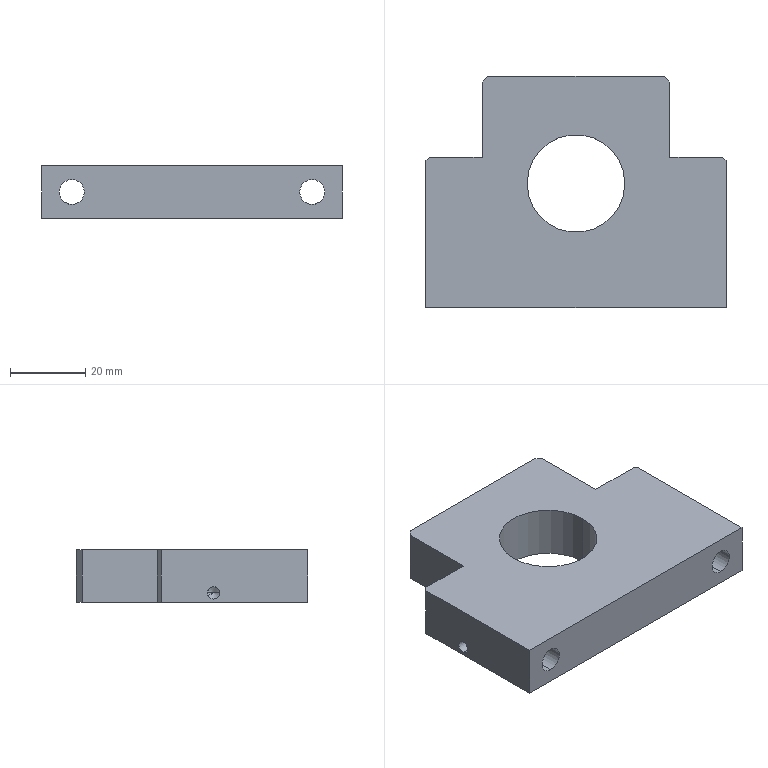Part | STEP file | 866-BDO024-93-03A | 1 solid | 42 faces | box 80 x 61.5 x 14 mm | volume 48551 mm3 | cylinder 18 | plane 16 | cone 8 | commonest cylinder face diameters 3.3 x8 6.6 x4 11 x4 26 x2
STEP:
#1=CARTESIAN_POINT('',(-13.,33.,7.));
#2=VERTEX_POINT('',#1);
#3=CARTESIAN_POINT('',(13.,33.,7.));
#4=VERTEX_POINT('',#3);
#5=CARTESIAN_POINT('',(0.,33.,7.));
#6=DIRECTION('',(0.,0.,1.));
#7=DIRECTION('',(-1.,0.,0.));
#8=AXIS2_PLACEMENT_3D('',#5,#6,#7);
#9=CIRCLE('',#8,13.);
#10=EDGE_CURVE('',#2,#4,#9,.T.);
#11=ORIENTED_EDGE('',*,*,#10,.T.);
#12=CARTESIAN_POINT('',(13.,33.,-7.));
#13=VERTEX_POINT('',#12);
#14=CARTESIAN_POINT('',(13.,33.,7.));
#15=DIRECTION('',(0.,0.,-1.));
#16=VECTOR('',#15,1000.);
#17=LINE('',#14,#16);
#18=EDGE_CURVE('',#4,#13,#17,.T.);
#19=ORIENTED_EDGE('',*,*,#18,.T.);
#20=CARTESIAN_POINT('',(-13.,33.,-7.));
#21=VERTEX_POINT('',#20);
#22=CARTESIAN_POINT('',(0.,33.,-7.));
#23=DIRECTION('',(0.,0.,1.));
#24=DIRECTION('',(-1.,0.,0.));
#25=AXIS2_PLACEMENT_3D('',#22,#23,#24);
#26=CIRCLE('',#25,13.);
#27=EDGE_CURVE('',#21,#13,#26,.T.);
#28=ORIENTED_EDGE('',*,*,#27,.F.);
#29=CARTESIAN_POINT('',(-13.,33.,7.));
#30=DIRECTION('',(0.,0.,-1.));
#31=VECTOR('',#30,1000.);
#32=LINE('',#29,#31);
#33=EDGE_CURVE('',#2,#21,#32,.T.);
#34=ORIENTED_EDGE('',*,*,#33,.F.);
#35=EDGE_LOOP('',(#11,#19,#28,#34));
#36=FACE_OUTER_BOUND('',#35,.T.);
#37=CARTESIAN_POINT('',(0.,33.,7.));
#38=DIRECTION('',(0.,0.,-1.));
#39=DIRECTION('',(-1.,0.,0.));
#40=AXIS2_PLACEMENT_3D('',#37,#38,#39);
#41=CYLINDRICAL_SURFACE('',#40,13.);
#42=ADVANCED_FACE('',(#36),#41,.F.);
#43=CARTESIAN_POINT('',(-15.,51.4,-1.65));
#44=VERTEX_POINT('',#43);
#45=CARTESIAN_POINT('',(-16.65,51.4,0.));
#46=VERTEX_POINT('',#45);
#47=CARTESIAN_POINT('',(-15.,51.4,0.));
#48=DIRECTION('',(0.,1.,0.));
#49=DIRECTION('',(0.,0.,1.));
#50=AXIS2_PLACEMENT_3D('',#47,#48,#49);
#51=CIRCLE('',#50,1.65);
#52=EDGE_CURVE('',#44,#46,#51,.T.);
#53=ORIENTED_EDGE('',*,*,#52,.F.);
#54=CARTESIAN_POINT('',(-15.,61.5,-1.65));
#55=VERTEX_POINT('',#54);
#56=CARTESIAN_POINT('',(-15.,61.5,-1.65));
#57=DIRECTION('',(0.,1.,0.));
#58=VECTOR('',#57,1000.);
#59=LINE('',#56,#58);
#60=EDGE_CURVE('',#44,#55,#59,.T.);
#61=ORIENTED_EDGE('',*,*,#60,.T.);
#62=CARTESIAN_POINT('',(-15.,61.5,1.65));
#63=VERTEX_POINT('',#62);
#64=CARTESIAN_POINT('',(-15.,61.5,0.));
#65=DIRECTION('',(0.,1.,0.));
#66=DIRECTION('',(0.,0.,1.));
#67=AXIS2_PLACEMENT_3D('',#64,#65,#66);
#68=CIRCLE('',#67,1.65);
#69=EDGE_CURVE('',#55,#63,#68,.T.);
#70=ORIENTED_EDGE('',*,*,#69,.T.);
#71=CARTESIAN_POINT('',(-15.,51.4,1.65));
#72=VERTEX_POINT('',#71);
#73=CARTESIAN_POINT('',(-15.,61.5,1.65));
#74=DIRECTION('',(0.,1.,0.));
#75=VECTOR('',#74,1000.);
#76=LINE('',#73,#75);
#77=EDGE_CURVE('',#72,#63,#76,.T.);
#78=ORIENTED_EDGE('',*,*,#77,.F.);
#79=CARTESIAN_POINT('',(-15.,51.4,0.));
#80=DIRECTION('',(0.,1.,0.));
#81=DIRECTION('',(0.,0.,1.));
#82=AXIS2_PLACEMENT_3D('',#79,#80,#81);
#83=CIRCLE('',#82,1.65);
#84=EDGE_CURVE('',#46,#72,#83,.T.);
#85=ORIENTED_EDGE('',*,*,#84,.F.);
#86=EDGE_LOOP('',(#53,#61,#70,#78,#85));
#87=FACE_OUTER_BOUND('',#86,.T.);
#88=CARTESIAN_POINT('',(-15.,61.5,0.));
#89=DIRECTION('',(0.,1.,0.));
#90=DIRECTION('',(0.,0.,1.));
#91=AXIS2_PLACEMENT_3D('',#88,#89,#90);
#92=CYLINDRICAL_SURFACE('',#91,1.65);
#93=ADVANCED_FACE('',(#87),#92,.F.);
#94=CARTESIAN_POINT('',(15.,51.4,-1.65));
#95=VERTEX_POINT('',#94);
#96=CARTESIAN_POINT('',(13.35,51.4,0.));
#97=VERTEX_POINT('',#96);
#98=CARTESIAN_POINT('',(15.,51.4,0.));
#99=DIRECTION('',(0.,1.,0.));
#100=DIRECTION('',(0.,0.,1.));
#101=AXIS2_PLACEMENT_3D('',#98,#99,#100);
#102=CIRCLE('',#101,1.65);
#103=EDGE_CURVE('',#95,#97,#102,.T.);
#104=ORIENTED_EDGE('',*,*,#103,.F.);
#105=CARTESIAN_POINT('',(15.,61.5,-1.65));
#106=VERTEX_POINT('',#105);
#107=CARTESIAN_POINT('',(15.,61.5,-1.65));
#108=DIRECTION('',(0.,1.,0.));
#109=VECTOR('',#108,1000.);
#110=LINE('',#107,#109);
#111=EDGE_CURVE('',#95,#106,#110,.T.);
#112=ORIENTED_EDGE('',*,*,#111,.T.);
#113=CARTESIAN_POINT('',(15.,61.5,1.65));
#114=VERTEX_POINT('',#113);
#115=CARTESIAN_POINT('',(15.,61.5,0.));
#116=DIRECTION('',(0.,1.,0.));
#117=DIRECTION('',(0.,0.,1.));
#118=AXIS2_PLACEMENT_3D('',#115,#116,#117);
#119=CIRCLE('',#118,1.65);
#120=EDGE_CURVE('',#106,#114,#119,.T.);
#121=ORIENTED_EDGE('',*,*,#120,.T.);
#122=CARTESIAN_POINT('',(15.,51.4,1.65));
#123=VERTEX_POINT('',#122);
#124=CARTESIAN_POINT('',(15.,61.5,1.65));
#125=DIRECTION('',(0.,1.,0.));
#126=VECTOR('',#125,1000.);
#127=LINE('',#124,#126);
#128=EDGE_CURVE('',#123,#114,#127,.T.);
#129=ORIENTED_EDGE('',*,*,#128,.F.);
#130=CARTESIAN_POINT('',(15.,51.4,0.));
#131=DIRECTION('',(0.,1.,0.));
#132=DIRECTION('',(0.,0.,1.));
#133=AXIS2_PLACEMENT_3D('',#130,#131,#132);
#134=CIRCLE('',#133,1.65);
#135=EDGE_CURVE('',#97,#123,#134,.T.);
#136=ORIENTED_EDGE('',*,*,#135,.F.);
#137=EDGE_LOOP('',(#104,#112,#121,#129,#136));
#138=FACE_OUTER_BOUND('',#137,.T.);
#139=CARTESIAN_POINT('',(15.,61.5,0.));
#140=DIRECTION('',(0.,1.,0.));
#141=DIRECTION('',(0.,0.,1.));
#142=AXIS2_PLACEMENT_3D('',#139,#140,#141);
#143=CYLINDRICAL_SURFACE('',#142,1.65);
#144=ADVANCED_FACE('',(#138),#143,.F.);
#145=CARTESIAN_POINT('',(-32.,34.,-5.5));
#146=VERTEX_POINT('',#145);
#147=CARTESIAN_POINT('',(-32.,34.,5.5));
#148=VERTEX_POINT('',#147);
#149=CARTESIAN_POINT('',(-32.,34.,0.));
#150=DIRECTION('',(0.,1.,0.));
#151=DIRECTION('',(0.,0.,1.));
#152=AXIS2_PLACEMENT_3D('',#149,#150,#151);
#153=CIRCLE('',#152,5.5);
#154=EDGE_CURVE('',#146,#148,#153,.T.);
#155=ORIENTED_EDGE('',*,*,#154,.F.);
#156=CARTESIAN_POINT('',(-32.,40.,-5.5));
#157=VERTEX_POINT('',#156);
#158=CARTESIAN_POINT('',(-32.,40.,-5.5));
#159=DIRECTION('',(0.,1.,0.));
#160=VECTOR('',#159,1000.);
#161=LINE('',#158,#160);
#162=EDGE_CURVE('',#146,#157,#161,.T.);
#163=ORIENTED_EDGE('',*,*,#162,.T.);
#164=CARTESIAN_POINT('',(-32.,40.,5.5));
#165=VERTEX_POINT('',#164);
#166=CARTESIAN_POINT('',(-32.,40.,0.));
#167=DIRECTION('',(0.,1.,0.));
#168=DIRECTION('',(0.,0.,1.));
#169=AXIS2_PLACEMENT_3D('',#166,#167,#168);
#170=CIRCLE('',#169,5.5);
#171=EDGE_CURVE('',#157,#165,#170,.T.);
#172=ORIENTED_EDGE('',*,*,#171,.T.);
#173=CARTESIAN_POINT('',(-32.,40.,5.5));
#174=DIRECTION('',(0.,1.,0.));
#175=VECTOR('',#174,1000.);
#176=LINE('',#173,#175);
#177=EDGE_CURVE('',#148,#165,#176,.T.);
#178=ORIENTED_EDGE('',*,*,#177,.F.);
#179=EDGE_LOOP('',(#155,#163,#172,#178));
#180=FACE_OUTER_BOUND('',#179,.T.);
#181=CARTESIAN_POINT('',(-32.,40.,0.));
#182=DIRECTION('',(0.,1.,0.));
#183=DIRECTION('',(0.,0.,1.));
#184=AXIS2_PLACEMENT_3D('',#181,#182,#183);
#185=CYLINDRICAL_SURFACE('',#184,5.5);
#186=ADVANCED_FACE('',(#180),#185,.F.);
#187=CARTESIAN_POINT('',(-29.9,25.,-6.15));
#188=VERTEX_POINT('',#187);
#189=CARTESIAN_POINT('',(-29.9,23.35,-4.5));
#190=VERTEX_POINT('',#189);
#191=CARTESIAN_POINT('',(-29.9,25.,-4.5));
#192=DIRECTION('',(-1.,0.,0.));
#193=DIRECTION('',(0.,0.,1.));
#194=AXIS2_PLACEMENT_3D('',#191,#192,#193);
#195=CIRCLE('',#194,1.65);
#196=EDGE_CURVE('',#188,#190,#195,.T.);
#197=ORIENTED_EDGE('',*,*,#196,.F.);
#198=CARTESIAN_POINT('',(-40.,25.,-6.15));
#199=VERTEX_POINT('',#198);
#200=CARTESIAN_POINT('',(-40.,25.,-6.15));
#201=DIRECTION('',(-1.,0.,0.));
#202=VECTOR('',#201,1000.);
#203=LINE('',#200,#202);
#204=EDGE_CURVE('',#188,#199,#203,.T.);
#205=ORIENTED_EDGE('',*,*,#204,.T.);
#206=CARTESIAN_POINT('',(-40.,25.,-2.85));
#207=VERTEX_POINT('',#206);
#208=CARTESIAN_POINT('',(-40.,25.,-4.5));
#209=DIRECTION('',(-1.,0.,0.));
#210=DIRECTION('',(0.,0.,1.));
#211=AXIS2_PLACEMENT_3D('',#208,#209,#210);
#212=CIRCLE('',#211,1.65);
#213=EDGE_CURVE('',#199,#207,#212,.T.);
#214=ORIENTED_EDGE('',*,*,#213,.T.);
#215=CARTESIAN_POINT('',(-33.664,25.,-2.85));
#216=VERTEX_POINT('',#215);
#217=CARTESIAN_POINT('',(-40.,25.,-2.85));
#218=DIRECTION('',(-1.,0.,0.));
#219=VECTOR('',#218,1000.);
#220=LINE('',#217,#219);
#221=EDGE_CURVE('',#216,#207,#220,.T.);
#222=ORIENTED_EDGE('',*,*,#221,.F.);
#223=CARTESIAN_POINT('',(-32.,23.868,-3.3));
#224=VERTEX_POINT('',#223);
#225=CARTESIAN_POINT('',(-32.,23.868,-3.3));
#226=CARTESIAN_POINT('',(-32.193,23.868,-3.3));
#227=CARTESIAN_POINT('',(-32.381,23.885,-3.283));
#228=CARTESIAN_POINT('',(-32.748,23.958,-3.219));
#229=CARTESIAN_POINT('',(-32.929,24.016,-3.171));
#230=CARTESIAN_POINT('',(-33.251,24.191,-3.058));
#231=CARTESIAN_POINT('',(-33.395,24.308,-2.993));
#232=CARTESIAN_POINT('',(-33.604,24.618,-2.886));
#233=CARTESIAN_POINT('',(-33.664,24.805,-2.85));
#234=CARTESIAN_POINT('',(-33.664,25.,-2.85));
#235=B_SPLINE_CURVE_WITH_KNOTS('',3,(#225,#226,#227,#228,#229,#230,#231,#232,#233,#234),.UNSPECIFIED.,.F.,.F.,(4,2,2,2,4),(0.004543,0.005111,0.005678,0.006246,0.006814),.UNSPECIFIED.);
#236=EDGE_CURVE('',#224,#216,#235,.T.);
#237=ORIENTED_EDGE('',*,*,#236,.F.);
#238=CARTESIAN_POINT('',(-30.336,25.,-2.85));
#239=VERTEX_POINT('',#238);
#240=CARTESIAN_POINT('',(-30.336,25.,-2.85));
#241=CARTESIAN_POINT('',(-30.336,24.903,-2.85));
#242=CARTESIAN_POINT('',(-30.351,24.809,-2.859));
#243=CARTESIAN_POINT('',(-30.407,24.627,-2.89));
#244=CARTESIAN_POINT('',(-30.448,24.542,-2.913));
#245=CARTESIAN_POINT('',(-30.603,24.311,-2.992));
#246=CARTESIAN_POINT('',(-30.747,24.192,-3.057));
#247=CARTESIAN_POINT('',(-31.069,24.017,-3.171));
#248=CARTESIAN_POINT('',(-31.247,23.959,-3.219));
#249=CARTESIAN_POINT('',(-31.618,23.884,-3.283));
#250=CARTESIAN_POINT('',(-31.807,23.868,-3.3));
#251=CARTESIAN_POINT('',(-32.,23.868,-3.3));
#252=B_SPLINE_CURVE_WITH_KNOTS('',3,(#240,#241,#242,#243,#244,#245,#246,#247,#248,#249,#250,#251),.UNSPECIFIED.,.F.,.F.,(4,2,2,2,2,4),(0.002272,0.002556,0.00284,0.003408,0.003975,0.004543),.UNSPECIFIED.);
#253=EDGE_CURVE('',#239,#224,#252,.T.);
#254=ORIENTED_EDGE('',*,*,#253,.F.);
#255=CARTESIAN_POINT('',(-29.9,25.,-2.85));
#256=VERTEX_POINT('',#255);
#257=CARTESIAN_POINT('',(-40.,25.,-2.85));
#258=DIRECTION('',(-1.,0.,0.));
#259=VECTOR('',#258,1000.);
#260=LINE('',#257,#259);
#261=EDGE_CURVE('',#256,#239,#260,.T.);
#262=ORIENTED_EDGE('',*,*,#261,.F.);
#263=CARTESIAN_POINT('',(-29.9,25.,-4.5));
#264=DIRECTION('',(-1.,0.,0.));
#265=DIRECTION('',(0.,0.,1.));
#266=AXIS2_PLACEMENT_3D('',#263,#264,#265);
#267=CIRCLE('',#266,1.65);
#268=EDGE_CURVE('',#190,#256,#267,.T.);
#269=ORIENTED_EDGE('',*,*,#268,.F.);
#270=EDGE_LOOP('',(#197,#205,#214,#222,#237,#254,#262,#269));
#271=FACE_OUTER_BOUND('',#270,.T.);
#272=CARTESIAN_POINT('',(-40.,25.,-4.5));
#273=DIRECTION('',(-1.,0.,0.));
#274=DIRECTION('',(0.,0.,1.));
#275=AXIS2_PLACEMENT_3D('',#272,#273,#274);
#276=CYLINDRICAL_SURFACE('',#275,1.65);
#277=ADVANCED_FACE('',(#271),#276,.F.);
#278=CARTESIAN_POINT('',(-32.,0.,3.3));
#279=VERTEX_POINT('',#278);
#280=CARTESIAN_POINT('',(-32.,0.,-3.3));
#281=VERTEX_POINT('',#280);
#282=CARTESIAN_POINT('',(-32.,0.,0.));
#283=DIRECTION('',(0.,-1.,0.));
#284=DIRECTION('',(0.,0.,1.));
#285=AXIS2_PLACEMENT_3D('',#282,#283,#284);
#286=CIRCLE('',#285,3.3);
#287=EDGE_CURVE('',#279,#281,#286,.T.);
#288=ORIENTED_EDGE('',*,*,#287,.T.);
#289=CARTESIAN_POINT('',(-32.,40.,-3.3));
#290=DIRECTION('',(0.,1.,0.));
#291=VECTOR('',#290,1000.);
#292=LINE('',#289,#291);
#293=EDGE_CURVE('',#281,#224,#292,.T.);
#294=ORIENTED_EDGE('',*,*,#293,.T.);
#295=ORIENTED_EDGE('',*,*,#236,.T.);
#296=CARTESIAN_POINT('',(-32.,26.132,-3.3));
#297=VERTEX_POINT('',#296);
#298=CARTESIAN_POINT('',(-33.664,25.,-2.85));
#299=CARTESIAN_POINT('',(-33.664,25.097,-2.85));
#300=CARTESIAN_POINT('',(-33.649,25.191,-2.859));
#301=CARTESIAN_POINT('',(-33.593,25.373,-2.89));
#302=CARTESIAN_POINT('',(-33.552,25.458,-2.913));
#303=CARTESIAN_POINT('',(-33.397,25.689,-2.992));
#304=CARTESIAN_POINT('',(-33.253,25.808,-3.057));
#305=CARTESIAN_POINT('',(-32.931,25.983,-3.171));
#306=CARTESIAN_POINT('',(-32.753,26.041,-3.219));
#307=CARTESIAN_POINT('',(-32.382,26.116,-3.283));
#308=CARTESIAN_POINT('',(-32.193,26.132,-3.3));
#309=CARTESIAN_POINT('',(-32.,26.132,-3.3));
#310=B_SPLINE_CURVE_WITH_KNOTS('',3,(#298,#299,#300,#301,#302,#303,#304,#305,#306,#307,#308,#309),.UNSPECIFIED.,.F.,.F.,(4,2,2,2,2,4),(-0.002271,-0.001987,-0.001703,-0.001136,-0.0005678,0.),.UNSPECIFIED.);
#311=EDGE_CURVE('',#216,#297,#310,.T.);
#312=ORIENTED_EDGE('',*,*,#311,.T.);
#313=CARTESIAN_POINT('',(-32.,34.,-3.3));
#314=VERTEX_POINT('',#313);
#315=CARTESIAN_POINT('',(-32.,40.,-3.3));
#316=DIRECTION('',(0.,1.,0.));
#317=VECTOR('',#316,1000.);
#318=LINE('',#315,#317);
#319=EDGE_CURVE('',#297,#314,#318,.T.);
#320=ORIENTED_EDGE('',*,*,#319,.T.);
#321=CARTESIAN_POINT('',(-32.,34.,3.3));
#322=VERTEX_POINT('',#321);
#323=CARTESIAN_POINT('',(-32.,34.,0.));
#324=DIRECTION('',(0.,-1.,0.));
#325=DIRECTION('',(0.,0.,1.));
#326=AXIS2_PLACEMENT_3D('',#323,#324,#325);
#327=CIRCLE('',#326,3.3);
#328=EDGE_CURVE('',#322,#314,#327,.T.);
#329=ORIENTED_EDGE('',*,*,#328,.F.);
#330=CARTESIAN_POINT('',(-32.,40.,3.3));
#331=DIRECTION('',(0.,1.,0.));
#332=VECTOR('',#331,1000.);
#333=LINE('',#330,#332);
#334=EDGE_CURVE('',#279,#322,#333,.T.);
#335=ORIENTED_EDGE('',*,*,#334,.F.);
#336=EDGE_LOOP('',(#288,#294,#295,#312,#320,#329,#335));
#337=FACE_OUTER_BOUND('',#336,.T.);
#338=CARTESIAN_POINT('',(-32.,40.,0.));
#339=DIRECTION('',(0.,1.,0.));
#340=DIRECTION('',(0.,0.,1.));
#341=AXIS2_PLACEMENT_3D('',#338,#339,#340);
#342=CYLINDRICAL_SURFACE('',#341,3.3);
#343=ADVANCED_FACE('',(#337),#342,.F.);
#344=CARTESIAN_POINT('',(32.,0.,3.3));
#345=VERTEX_POINT('',#344);
#346=CARTESIAN_POINT('',(32.,0.,-3.3));
#347=VERTEX_POINT('',#346);
#348=CARTESIAN_POINT('',(32.,0.,0.));
#349=DIRECTION('',(0.,-1.,0.));
#350=DIRECTION('',(0.,0.,1.));
#351=AXIS2_PLACEMENT_3D('',#348,#349,#350);
#352=CIRCLE('',#351,3.3);
#353=EDGE_CURVE('',#345,#347,#352,.T.);
#354=ORIENTED_EDGE('',*,*,#353,.T.);
#355=CARTESIAN_POINT('',(32.,23.868,-3.3));
#356=VERTEX_POINT('',#355);
#357=CARTESIAN_POINT('',(32.,40.,-3.3));
#358=DIRECTION('',(0.,1.,0.));
#359=VECTOR('',#358,1000.);
#360=LINE('',#357,#359);
#361=EDGE_CURVE('',#347,#356,#360,.T.);
#362=ORIENTED_EDGE('',*,*,#361,.T.);
#363=CARTESIAN_POINT('',(30.336,25.,-2.85));
#364=VERTEX_POINT('',#363);
#365=CARTESIAN_POINT('',(30.336,25.,-2.85));
#366=CARTESIAN_POINT('',(30.336,24.903,-2.85));
#367=CARTESIAN_POINT('',(30.351,24.809,-2.859));
#368=CARTESIAN_POINT('',(30.407,24.627,-2.89));
#369=CARTESIAN_POINT('',(30.448,24.542,-2.913));
#370=CARTESIAN_POINT('',(30.603,24.311,-2.992));
#371=CARTESIAN_POINT('',(30.747,24.192,-3.057));
#372=CARTESIAN_POINT('',(31.069,24.017,-3.171));
#373=CARTESIAN_POINT('',(31.247,23.959,-3.219));
#374=CARTESIAN_POINT('',(31.618,23.884,-3.283));
#375=CARTESIAN_POINT('',(31.807,23.868,-3.3));
#376=CARTESIAN_POINT('',(32.,23.868,-3.3));
#377=B_SPLINE_CURVE_WITH_KNOTS('',3,(#365,#366,#367,#368,#369,#370,#371,#372,#373,#374,#375,#376),.UNSPECIFIED.,.F.,.F.,(4,2,2,2,2,4),(0.004583,0.004869,0.005155,0.005728,0.0063,0.006873),.UNSPECIFIED.);
#378=EDGE_CURVE('',#364,#356,#377,.T.);
#379=ORIENTED_EDGE('',*,*,#378,.F.);
#380=CARTESIAN_POINT('',(32.,26.132,-3.3));
#381=VERTEX_POINT('',#380);
#382=CARTESIAN_POINT('',(32.,26.132,-3.3));
#383=CARTESIAN_POINT('',(31.807,26.132,-3.3));
#384=CARTESIAN_POINT('',(31.619,26.115,-3.283));
#385=CARTESIAN_POINT('',(31.252,26.042,-3.219));
#386=CARTESIAN_POINT('',(31.071,25.984,-3.171));
#387=CARTESIAN_POINT('',(30.749,25.809,-3.058));
#388=CARTESIAN_POINT('',(30.605,25.692,-2.993));
#389=CARTESIAN_POINT('',(30.396,25.382,-2.886));
#390=CARTESIAN_POINT('',(30.336,25.195,-2.85));
#391=CARTESIAN_POINT('',(30.336,25.,-2.85));
#392=B_SPLINE_CURVE_WITH_KNOTS('',3,(#382,#383,#384,#385,#386,#387,#388,#389,#390,#391),.UNSPECIFIED.,.F.,.F.,(4,2,2,2,4),(0.002291,0.002864,0.003437,0.00401,0.004583),.UNSPECIFIED.);
#393=EDGE_CURVE('',#381,#364,#392,.T.);
#394=ORIENTED_EDGE('',*,*,#393,.F.);
#395=CARTESIAN_POINT('',(32.,34.,-3.3));
#396=VERTEX_POINT('',#395);
#397=CARTESIAN_POINT('',(32.,40.,-3.3));
#398=DIRECTION('',(0.,1.,0.));
#399=VECTOR('',#398,1000.);
#400=LINE('',#397,#399);
#401=EDGE_CURVE('',#381,#396,#400,.T.);
#402=ORIENTED_EDGE('',*,*,#401,.T.);
#403=CARTESIAN_POINT('',(32.,34.,3.3));
#404=VERTEX_POINT('',#403);
#405=CARTESIAN_POINT('',(32.,34.,0.));
#406=DIRECTION('',(0.,-1.,0.));
#407=DIRECTION('',(0.,0.,1.));
#408=AXIS2_PLACEMENT_3D('',#405,#406,#407);
#409=CIRCLE('',#408,3.3);
#410=EDGE_CURVE('',#404,#396,#409,.T.);
#411=ORIENTED_EDGE('',*,*,#410,.F.);
#412=CARTESIAN_POINT('',(32.,40.,3.3));
#413=DIRECTION('',(0.,1.,0.));
#414=VECTOR('',#413,1000.);
#415=LINE('',#412,#414);
#416=EDGE_CURVE('',#345,#404,#415,.T.);
#417=ORIENTED_EDGE('',*,*,#416,.F.);
#418=EDGE_LOOP('',(#354,#362,#379,#394,#402,#411,#417));
#419=FACE_OUTER_BOUND('',#418,.T.);
#420=CARTESIAN_POINT('',(32.,40.,0.));
#421=DIRECTION('',(0.,1.,0.));
#422=DIRECTION('',(0.,0.,1.));
#423=AXIS2_PLACEMENT_3D('',#420,#421,#422);
#424=CYLINDRICAL_SURFACE('',#423,3.3);
#425=ADVANCED_FACE('',(#419),#424,.F.);
#426=CARTESIAN_POINT('',(29.9,25.,-2.85));
#427=VERTEX_POINT('',#426);
#428=CARTESIAN_POINT('',(29.9,25.,-6.15));
#429=VERTEX_POINT('',#428);
#430=CARTESIAN_POINT('',(29.9,25.,-4.5));
#431=DIRECTION('',(1.,0.,0.));
#432=DIRECTION('',(0.,0.,-1.));
#433=AXIS2_PLACEMENT_3D('',#430,#431,#432);
#434=CIRCLE('',#433,1.65);
#435=EDGE_CURVE('',#427,#429,#434,.T.);
#436=ORIENTED_EDGE('',*,*,#435,.F.);
#437=CARTESIAN_POINT('',(40.,25.,-2.85));
#438=DIRECTION('',(1.,0.,0.));
#439=VECTOR('',#438,1000.);
#440=LINE('',#437,#439);
#441=EDGE_CURVE('',#427,#364,#440,.T.);
#442=ORIENTED_EDGE('',*,*,#441,.T.);
#443=ORIENTED_EDGE('',*,*,#378,.T.);
#444=CARTESIAN_POINT('',(33.664,25.,-2.85));
#445=VERTEX_POINT('',#444);
#446=CARTESIAN_POINT('',(32.,23.868,-3.3));
#447=CARTESIAN_POINT('',(32.193,23.868,-3.3));
#448=CARTESIAN_POINT('',(32.381,23.885,-3.283));
#449=CARTESIAN_POINT('',(32.748,23.958,-3.219));
#450=CARTESIAN_POINT('',(32.929,24.016,-3.171));
#451=CARTESIAN_POINT('',(33.251,24.191,-3.058));
#452=CARTESIAN_POINT('',(33.395,24.308,-2.993));
#453=CARTESIAN_POINT('',(33.604,24.618,-2.886));
#454=CARTESIAN_POINT('',(33.664,24.805,-2.85));
#455=CARTESIAN_POINT('',(33.664,25.,-2.85));
#456=B_SPLINE_CURVE_WITH_KNOTS('',3,(#446,#447,#448,#449,#450,#451,#452,#453,#454,#455),.UNSPECIFIED.,.F.,.F.,(4,2,2,2,4),(-0.002293,-0.00172,-0.001146,-0.0005732,0.),.UNSPECIFIED.);
#457=EDGE_CURVE('',#356,#445,#456,.T.);
#458=ORIENTED_EDGE('',*,*,#457,.T.);
#459=CARTESIAN_POINT('',(40.,25.,-2.85));
#460=VERTEX_POINT('',#459);
#461=CARTESIAN_POINT('',(40.,25.,-2.85));
#462=DIRECTION('',(1.,0.,0.));
#463=VECTOR('',#462,1000.);
#464=LINE('',#461,#463);
#465=EDGE_CURVE('',#445,#460,#464,.T.);
#466=ORIENTED_EDGE('',*,*,#465,.T.);
#467=CARTESIAN_POINT('',(40.,25.,-6.15));
#468=VERTEX_POINT('',#467);
#469=CARTESIAN_POINT('',(40.,25.,-4.5));
#470=DIRECTION('',(1.,0.,0.));
#471=DIRECTION('',(0.,0.,-1.));
#472=AXIS2_PLACEMENT_3D('',#469,#470,#471);
#473=CIRCLE('',#472,1.65);
#474=EDGE_CURVE('',#460,#468,#473,.T.);
#475=ORIENTED_EDGE('',*,*,#474,.T.);
#476=CARTESIAN_POINT('',(40.,25.,-6.15));
#477=DIRECTION('',(1.,0.,0.));
#478=VECTOR('',#477,1000.);
#479=LINE('',#476,#478);
#480=EDGE_CURVE('',#429,#468,#479,.T.);
#481=ORIENTED_EDGE('',*,*,#480,.F.);
#482=EDGE_LOOP('',(#436,#442,#443,#458,#466,#475,#481));
#483=FACE_OUTER_BOUND('',#482,.T.);
#484=CARTESIAN_POINT('',(40.,25.,-4.5));
#485=DIRECTION('',(1.,0.,0.));
#486=DIRECTION('',(0.,0.,-1.));
#487=AXIS2_PLACEMENT_3D('',#484,#485,#486);
#488=CYLINDRICAL_SURFACE('',#487,1.65);
#489=ADVANCED_FACE('',(#483),#488,.F.);
#490=CARTESIAN_POINT('',(32.,34.,-5.5));
#491=VERTEX_POINT('',#490);
#492=CARTESIAN_POINT('',(32.,34.,5.5));
#493=VERTEX_POINT('',#492);
#494=CARTESIAN_POINT('',(32.,34.,0.));
#495=DIRECTION('',(0.,1.,0.));
#496=DIRECTION('',(0.,0.,1.));
#497=AXIS2_PLACEMENT_3D('',#494,#495,#496);
#498=CIRCLE('',#497,5.5);
#499=EDGE_CURVE('',#491,#493,#498,.T.);
#500=ORIENTED_EDGE('',*,*,#499,.F.);
#501=CARTESIAN_POINT('',(32.,40.,-5.5));
#502=VERTEX_POINT('',#501);
#503=CARTESIAN_POINT('',(32.,40.,-5.5));
#504=DIRECTION('',(0.,1.,0.));
#505=VECTOR('',#504,1000.);
#506=LINE('',#503,#505);
#507=EDGE_CURVE('',#491,#502,#506,.T.);
#508=ORIENTED_EDGE('',*,*,#507,.T.);
#509=CARTESIAN_POINT('',(32.,40.,5.5));
#510=VERTEX_POINT('',#509);
#511=CARTESIAN_POINT('',(32.,40.,0.));
#512=DIRECTION('',(0.,1.,0.));
#513=DIRECTION('',(0.,0.,1.));
#514=AXIS2_PLACEMENT_3D('',#511,#512,#513);
#515=CIRCLE('',#514,5.5);
#516=EDGE_CURVE('',#502,#510,#515,.T.);
#517=ORIENTED_EDGE('',*,*,#516,.T.);
#518=CARTESIAN_POINT('',(32.,40.,5.5));
#519=DIRECTION('',(0.,1.,0.));
#520=VECTOR('',#519,1000.);
#521=LINE('',#518,#520);
#522=EDGE_CURVE('',#493,#510,#521,.T.);
#523=ORIENTED_EDGE('',*,*,#522,.F.);
#524=EDGE_LOOP('',(#500,#508,#517,#523));
#525=FACE_OUTER_BOUND('',#524,.T.);
#526=CARTESIAN_POINT('',(32.,40.,0.));
#527=DIRECTION('',(0.,1.,0.));
#528=DIRECTION('',(0.,0.,1.));
#529=AXIS2_PLACEMENT_3D('',#526,#527,#528);
#530=CYLINDRICAL_SURFACE('',#529,5.5);
#531=ADVANCED_FACE('',(#525),#530,.F.);
#532=CARTESIAN_POINT('',(-15.,50.409,0.));
#533=VERTEX_POINT('',#532);
#534=CARTESIAN_POINT('',(-16.65,51.4,0.));
#535=DIRECTION('',(-0.8572,0.515,0.));
#536=VECTOR('',#535,1000.);
#537=LINE('',#534,#536);
#538=EDGE_CURVE('',#533,#46,#537,.T.);
#539=ORIENTED_EDGE('',*,*,#538,.F.);
#540=CARTESIAN_POINT('',(-13.35,51.4,0.));
#541=VERTEX_POINT('',#540);
#542=CARTESIAN_POINT('',(-13.35,51.4,0.));
#543=DIRECTION('',(0.8572,0.515,0.));
#544=VECTOR('',#543,1000.);
#545=LINE('',#542,#544);
#546=EDGE_CURVE('',#533,#541,#545,.T.);
#547=ORIENTED_EDGE('',*,*,#546,.T.);
#548=CARTESIAN_POINT('',(-15.,51.4,0.));
#549=DIRECTION('',(0.,1.,0.));
#550=DIRECTION('',(0.,0.,1.));
#551=AXIS2_PLACEMENT_3D('',#548,#549,#550);
#552=CIRCLE('',#551,1.65);
#553=EDGE_CURVE('',#541,#44,#552,.T.);
#554=ORIENTED_EDGE('',*,*,#553,.T.);
#555=ORIENTED_EDGE('',*,*,#52,.T.);
#556=EDGE_LOOP('',(#539,#547,#554,#555));
#557=FACE_OUTER_BOUND('',#556,.T.);
#558=CARTESIAN_POINT('',(-15.,51.4,0.));
#559=DIRECTION('',(0.,1.,0.));
#560=DIRECTION('',(-1.,0.,0.));
#561=AXIS2_PLACEMENT_3D('',#558,#559,#560);
#562=CONICAL_SURFACE('',#561,1.65,1.03);
#563=ADVANCED_FACE('',(#557),#562,.F.);
#564=CARTESIAN_POINT('',(15.,50.409,0.));
#565=VERTEX_POINT('',#564);
#566=CARTESIAN_POINT('',(13.35,51.4,0.));
#567=DIRECTION('',(-0.8572,0.515,0.));
#568=VECTOR('',#567,1000.);
#569=LINE('',#566,#568);
#570=EDGE_CURVE('',#565,#97,#569,.T.);
#571=ORIENTED_EDGE('',*,*,#570,.F.);
#572=CARTESIAN_POINT('',(16.65,51.4,0.));
#573=VERTEX_POINT('',#572);
#574=CARTESIAN_POINT('',(16.65,51.4,0.));
#575=DIRECTION('',(0.8572,0.515,0.));
#576=VECTOR('',#575,1000.);
#577=LINE('',#574,#576);
#578=EDGE_CURVE('',#565,#573,#577,.T.);
#579=ORIENTED_EDGE('',*,*,#578,.T.);
#580=CARTESIAN_POINT('',(15.,51.4,0.));
#581=DIRECTION('',(0.,1.,0.));
#582=DIRECTION('',(0.,0.,1.));
#583=AXIS2_PLACEMENT_3D('',#580,#581,#582);
#584=CIRCLE('',#583,1.65);
#585=EDGE_CURVE('',#573,#95,#584,.T.);
#586=ORIENTED_EDGE('',*,*,#585,.T.);
#587=ORIENTED_EDGE('',*,*,#103,.T.);
#588=EDGE_LOOP('',(#571,#579,#586,#587));
#589=FACE_OUTER_BOUND('',#588,.T.);
#590=CARTESIAN_POINT('',(15.,51.4,0.));
#591=DIRECTION('',(0.,1.,0.));
#592=DIRECTION('',(-1.,0.,0.));
#593=AXIS2_PLACEMENT_3D('',#590,#591,#592);
#594=CONICAL_SURFACE('',#593,1.65,1.03);
#595=ADVANCED_FACE('',(#589),#594,.F.);
#596=CARTESIAN_POINT('',(-28.909,25.,-4.5));
#597=VERTEX_POINT('',#596);
#598=CARTESIAN_POINT('',(-29.9,23.35,-4.5));
#599=DIRECTION('',(-0.515,-0.8572,0.));
#600=VECTOR('',#599,1000.);
#601=LINE('',#598,#600);
#602=EDGE_CURVE('',#597,#190,#601,.T.);
#603=ORIENTED_EDGE('',*,*,#602,.F.);
#604=CARTESIAN_POINT('',(-29.9,26.65,-4.5));
#605=VERTEX_POINT('',#604);
#606=CARTESIAN_POINT('',(-29.9,26.65,-4.5));
#607=DIRECTION('',(-0.515,0.8572,0.));
#608=VECTOR('',#607,1000.);
#609=LINE('',#606,#608);
#610=EDGE_CURVE('',#597,#605,#609,.T.);
#611=ORIENTED_EDGE('',*,*,#610,.T.);
#612=CARTESIAN_POINT('',(-29.9,25.,-4.5));
#613=DIRECTION('',(-1.,0.,0.));
#614=DIRECTION('',(0.,0.,1.));
#615=AXIS2_PLACEMENT_3D('',#612,#613,#614);
#616=CIRCLE('',#615,1.65);
#617=EDGE_CURVE('',#605,#188,#616,.T.);
#618=ORIENTED_EDGE('',*,*,#617,.T.);
#619=ORIENTED_EDGE('',*,*,#196,.T.);
#620=EDGE_LOOP('',(#603,#611,#618,#619));
#621=FACE_OUTER_BOUND('',#620,.T.);
#622=CARTESIAN_POINT('',(-29.9,25.,-4.5));
#623=DIRECTION('',(-1.,0.,0.));
#624=DIRECTION('',(0.,-1.,0.));
#625=AXIS2_PLACEMENT_3D('',#622,#623,#624);
#626=CONICAL_SURFACE('',#625,1.65,1.03);
#627=ADVANCED_FACE('',(#621),#626,.F.);
#628=CARTESIAN_POINT('',(28.909,25.,-4.5));
#629=VERTEX_POINT('',#628);
#630=CARTESIAN_POINT('',(29.9,25.,-6.15));
#631=DIRECTION('',(0.515,0.,-0.8572));
#632=VECTOR('',#631,1000.);
#633=LINE('',#630,#632);
#634=EDGE_CURVE('',#629,#429,#633,.T.);
#635=ORIENTED_EDGE('',*,*,#634,.F.);
#636=CARTESIAN_POINT('',(29.9,25.,-2.85));
#637=DIRECTION('',(0.515,0.,0.8572));
#638=VECTOR('',#637,1000.);
#639=LINE('',#636,#638);
#640=EDGE_CURVE('',#629,#427,#639,.T.);
#641=ORIENTED_EDGE('',*,*,#640,.T.);
#642=ORIENTED_EDGE('',*,*,#435,.T.);
#643=EDGE_LOOP('',(#635,#641,#642));
#644=FACE_OUTER_BOUND('',#643,.T.);
#645=CARTESIAN_POINT('',(29.9,25.,-4.5));
#646=DIRECTION('',(1.,0.,0.));
#647=DIRECTION('',(0.,0.,-1.));
#648=AXIS2_PLACEMENT_3D('',#645,#646,#647);
#649=CONICAL_SURFACE('',#648,1.65,1.03);
#650=ADVANCED_FACE('',(#644),#649,.F.);
#651=ORIENTED_EDGE('',*,*,#10,.F.);
#652=CARTESIAN_POINT('',(0.,33.,7.));
#653=DIRECTION('',(0.,0.,1.));
#654=DIRECTION('',(-1.,0.,0.));
#655=AXIS2_PLACEMENT_3D('',#652,#653,#654);
#656=CIRCLE('',#655,13.);
#657=EDGE_CURVE('',#4,#2,#656,.T.);
#658=ORIENTED_EDGE('',*,*,#657,.F.);
#659=EDGE_LOOP('',(#651,#658));
#660=FACE_BOUND('',#659,.T.);
#661=CARTESIAN_POINT('',(23.5,61.5,7.));
#662=VERTEX_POINT('',#661);
#663=CARTESIAN_POINT('',(25.,60.,7.));
#664=VERTEX_POINT('',#663);
#665=CARTESIAN_POINT('',(23.5,61.5,7.));
#666=DIRECTION('',(0.7071,-0.7071,0.));
#667=VECTOR('',#666,1000.);
#668=LINE('',#665,#667);
#669=EDGE_CURVE('',#662,#664,#668,.T.);
#670=ORIENTED_EDGE('',*,*,#669,.F.);
#671=CARTESIAN_POINT('',(-23.5,61.5,7.));
#672=VERTEX_POINT('',#671);
#673=CARTESIAN_POINT('',(-40.,61.5,7.));
#674=DIRECTION('',(1.,0.,0.));
#675=VECTOR('',#674,1000.);
#676=LINE('',#673,#675);
#677=EDGE_CURVE('',#672,#662,#676,.T.);
#678=ORIENTED_EDGE('',*,*,#677,.F.);
#679=CARTESIAN_POINT('',(-25.,60.,7.));
#680=VERTEX_POINT('',#679);
#681=CARTESIAN_POINT('',(-25.,60.,7.));
#682=DIRECTION('',(0.7071,0.7071,0.));
#683=VECTOR('',#682,1000.);
#684=LINE('',#681,#683);
#685=EDGE_CURVE('',#680,#672,#684,.T.);
#686=ORIENTED_EDGE('',*,*,#685,.F.);
#687=CARTESIAN_POINT('',(-25.,40.,7.));
#688=VERTEX_POINT('',#687);
#689=CARTESIAN_POINT('',(-25.,40.,7.));
#690=DIRECTION('',(0.,1.,0.));
#691=VECTOR('',#690,1000.);
#692=LINE('',#689,#691);
#693=EDGE_CURVE('',#688,#680,#692,.T.);
#694=ORIENTED_EDGE('',*,*,#693,.F.);
#695=CARTESIAN_POINT('',(-39.,40.,7.));
#696=VERTEX_POINT('',#695);
#697=CARTESIAN_POINT('',(-40.,40.,7.));
#698=DIRECTION('',(1.,0.,0.));
#699=VECTOR('',#698,1000.);
#700=LINE('',#697,#699);
#701=EDGE_CURVE('',#696,#688,#700,.T.);
#702=ORIENTED_EDGE('',*,*,#701,.F.);
#703=CARTESIAN_POINT('',(-40.,39.,7.));
#704=VERTEX_POINT('',#703);
#705=CARTESIAN_POINT('',(-40.,39.,7.));
#706=DIRECTION('',(-0.7071,-0.7071,0.));
#707=VECTOR('',#706,1000.);
#708=LINE('',#705,#707);
#709=EDGE_CURVE('',#696,#704,#708,.T.);
#710=ORIENTED_EDGE('',*,*,#709,.T.);
#711=CARTESIAN_POINT('',(-40.,0.,7.));
#712=VERTEX_POINT('',#711);
#713=CARTESIAN_POINT('',(-40.,40.,7.));
#714=DIRECTION('',(0.,1.,0.));
#715=VECTOR('',#714,1000.);
#716=LINE('',#713,#715);
#717=EDGE_CURVE('',#712,#704,#716,.T.);
#718=ORIENTED_EDGE('',*,*,#717,.F.);
#719=CARTESIAN_POINT('',(40.,0.,7.));
#720=VERTEX_POINT('',#719);
#721=CARTESIAN_POINT('',(-40.,0.,7.));
#722=DIRECTION('',(-1.,0.,0.));
#723=VECTOR('',#722,1000.);
#724=LINE('',#721,#723);
#725=EDGE_CURVE('',#720,#712,#724,.T.);
#726=ORIENTED_EDGE('',*,*,#725,.F.);
#727=CARTESIAN_POINT('',(40.,39.,7.));
#728=VERTEX_POINT('',#727);
#729=CARTESIAN_POINT('',(40.,40.,7.));
#730=DIRECTION('',(0.,-1.,0.));
#731=VECTOR('',#730,1000.);
#732=LINE('',#729,#731);
#733=EDGE_CURVE('',#728,#720,#732,.T.);
#734=ORIENTED_EDGE('',*,*,#733,.F.);
#735=CARTESIAN_POINT('',(39.,40.,7.));
#736=VERTEX_POINT('',#735);
#737=CARTESIAN_POINT('',(39.,40.,7.));
#738=DIRECTION('',(-0.7071,0.7071,0.));
#739=VECTOR('',#738,1000.);
#740=LINE('',#737,#739);
#741=EDGE_CURVE('',#728,#736,#740,.T.);
#742=ORIENTED_EDGE('',*,*,#741,.T.);
#743=CARTESIAN_POINT('',(25.,40.,7.));
#744=VERTEX_POINT('',#743);
#745=CARTESIAN_POINT('',(-40.,40.,7.));
#746=DIRECTION('',(1.,0.,0.));
#747=VECTOR('',#746,1000.);
#748=LINE('',#745,#747);
#749=EDGE_CURVE('',#744,#736,#748,.T.);
#750=ORIENTED_EDGE('',*,*,#749,.F.);
#751=CARTESIAN_POINT('',(25.,40.,7.));
#752=DIRECTION('',(0.,-1.,0.));
#753=VECTOR('',#752,1000.);
#754=LINE('',#751,#753);
#755=EDGE_CURVE('',#664,#744,#754,.T.);
#756=ORIENTED_EDGE('',*,*,#755,.F.);
#757=EDGE_LOOP('',(#670,#678,#686,#694,#702,#710,#718,#726,#734,#742,#750,#756));
#758=FACE_OUTER_BOUND('',#757,.T.);
#759=CARTESIAN_POINT('',(-40.,40.,7.));
#760=DIRECTION('',(0.,0.,-1.));
#761=DIRECTION('',(-1.,0.,0.));
#762=AXIS2_PLACEMENT_3D('',#759,#760,#761);
#763=PLANE('',#762);
#764=ADVANCED_FACE('',(#660,#758),#763,.F.);
#765=ORIENTED_EDGE('',*,*,#18,.F.);
#766=ORIENTED_EDGE('',*,*,#657,.T.);
#767=ORIENTED_EDGE('',*,*,#33,.T.);
#768=CARTESIAN_POINT('',(0.,33.,-7.));
#769=DIRECTION('',(0.,0.,1.));
#770=DIRECTION('',(-1.,0.,0.));
#771=AXIS2_PLACEMENT_3D('',#768,#769,#770);
#772=CIRCLE('',#771,13.);
#773=EDGE_CURVE('',#13,#21,#772,.T.);
#774=ORIENTED_EDGE('',*,*,#773,.F.);
#775=EDGE_LOOP('',(#765,#766,#767,#774));
#776=FACE_OUTER_BOUND('',#775,.T.);
#777=CARTESIAN_POINT('',(0.,33.,7.));
#778=DIRECTION('',(0.,0.,-1.));
#779=DIRECTION('',(-1.,0.,0.));
#780=AXIS2_PLACEMENT_3D('',#777,#778,#779);
#781=CYLINDRICAL_SURFACE('',#780,13.);
#782=ADVANCED_FACE('',(#776),#781,.F.);
#783=CARTESIAN_POINT('',(25.,60.,-7.));
#784=VERTEX_POINT('',#783);
#785=CARTESIAN_POINT('',(25.,60.,7.));
#786=DIRECTION('',(0.,0.,-1.));
#787=VECTOR('',#786,1000.);
#788=LINE('',#785,#787);
#789=EDGE_CURVE('',#664,#784,#788,.T.);
#790=ORIENTED_EDGE('',*,*,#789,.F.);
#791=ORIENTED_EDGE('',*,*,#755,.T.);
#792=CARTESIAN_POINT('',(25.,40.,-7.));
#793=VERTEX_POINT('',#792);
#794=CARTESIAN_POINT('',(25.,40.,7.));
#795=DIRECTION('',(0.,0.,1.));
#796=VECTOR('',#795,1000.);
#797=LINE('',#794,#796);
#798=EDGE_CURVE('',#793,#744,#797,.T.);
#799=ORIENTED_EDGE('',*,*,#798,.F.);
#800=CARTESIAN_POINT('',(25.,61.5,-7.));
#801=DIRECTION('',(0.,-1.,0.));
#802=VECTOR('',#801,1000.);
#803=LINE('',#800,#802);
#804=EDGE_CURVE('',#784,#793,#803,.T.);
#805=ORIENTED_EDGE('',*,*,#804,.F.);
#806=EDGE_LOOP('',(#790,#791,#799,#805));
#807=FACE_OUTER_BOUND('',#806,.T.);
#808=CARTESIAN_POINT('',(25.,61.5,7.));
#809=DIRECTION('',(-1.,0.,0.));
#810=DIRECTION('',(0.,-1.,0.));
#811=AXIS2_PLACEMENT_3D('',#808,#809,#810);
#812=PLANE('',#811);
#813=ADVANCED_FACE('',(#807),#812,.F.);
#814=ORIENTED_EDGE('',*,*,#789,.T.);
#815=CARTESIAN_POINT('',(23.5,61.5,-7.));
#816=VERTEX_POINT('',#815);
#817=CARTESIAN_POINT('',(23.5,61.5,-7.));
#818=DIRECTION('',(0.7071,-0.7071,0.));
#819=VECTOR('',#818,1000.);
#820=LINE('',#817,#819);
#821=EDGE_CURVE('',#816,#784,#820,.T.);
#822=ORIENTED_EDGE('',*,*,#821,.F.);
#823=CARTESIAN_POINT('',(23.5,61.5,7.));
#824=DIRECTION('',(0.,0.,-1.));
#825=VECTOR('',#824,1000.);
#826=LINE('',#823,#825);
#827=EDGE_CURVE('',#662,#816,#826,.T.);
#828=ORIENTED_EDGE('',*,*,#827,.F.);
#829=ORIENTED_EDGE('',*,*,#669,.T.);
#830=EDGE_LOOP('',(#814,#822,#828,#829));
#831=FACE_OUTER_BOUND('',#830,.T.);
#832=CARTESIAN_POINT('',(23.5,61.5,7.));
#833=DIRECTION('',(-0.7071,-0.7071,0.));
#834=DIRECTION('',(0.7071,-0.7071,0.));
#835=AXIS2_PLACEMENT_3D('',#832,#833,#834);
#836=PLANE('',#835);
#837=ADVANCED_FACE('',(#831),#836,.F.);
#838=ORIENTED_EDGE('',*,*,#827,.T.);
#839=CARTESIAN_POINT('',(-23.5,61.5,-7.));
#840=VERTEX_POINT('',#839);
#841=CARTESIAN_POINT('',(-25.,61.5,-7.));
#842=DIRECTION('',(1.,0.,0.));
#843=VECTOR('',#842,1000.);
#844=LINE('',#841,#843);
#845=EDGE_CURVE('',#840,#816,#844,.T.);
#846=ORIENTED_EDGE('',*,*,#845,.F.);
#847=CARTESIAN_POINT('',(-23.5,61.5,7.));
#848=DIRECTION('',(0.,0.,-1.));
#849=VECTOR('',#848,1000.);
#850=LINE('',#847,#849);
#851=EDGE_CURVE('',#672,#840,#850,.T.);
#852=ORIENTED_EDGE('',*,*,#851,.F.);
#853=ORIENTED_EDGE('',*,*,#677,.T.);
#854=EDGE_LOOP('',(#838,#846,#852,#853));
#855=FACE_OUTER_BOUND('',#854,.T.);
#856=CARTESIAN_POINT('',(-15.,61.5,0.));
#857=DIRECTION('',(0.,1.,0.));
#858=DIRECTION('',(0.,0.,1.));
#859=AXIS2_PLACEMENT_3D('',#856,#857,#858);
#860=CIRCLE('',#859,1.65);
#861=EDGE_CURVE('',#63,#55,#860,.T.);
#862=ORIENTED_EDGE('',*,*,#861,.F.);
#863=ORIENTED_EDGE('',*,*,#69,.F.);
#864=EDGE_LOOP('',(#862,#863));
#865=FACE_BOUND('',#864,.T.);
#866=CARTESIAN_POINT('',(15.,61.5,0.));
#867=DIRECTION('',(0.,1.,0.));
#868=DIRECTION('',(0.,0.,1.));
#869=AXIS2_PLACEMENT_3D('',#866,#867,#868);
#870=CIRCLE('',#869,1.65);
#871=EDGE_CURVE('',#114,#106,#870,.T.);
#872=ORIENTED_EDGE('',*,*,#871,.F.);
#873=ORIENTED_EDGE('',*,*,#120,.F.);
#874=EDGE_LOOP('',(#872,#873));
#875=FACE_BOUND('',#874,.T.);
#876=CARTESIAN_POINT('',(-25.,61.5,7.));
#877=DIRECTION('',(0.,-1.,0.));
#878=DIRECTION('',(0.,0.,-1.));
#879=AXIS2_PLACEMENT_3D('',#876,#877,#878);
#880=PLANE('',#879);
#881=ADVANCED_FACE('',(#855,#865,#875),#880,.F.);
#882=ORIENTED_EDGE('',*,*,#851,.T.);
#883=CARTESIAN_POINT('',(-25.,60.,-7.));
#884=VERTEX_POINT('',#883);
#885=CARTESIAN_POINT('',(-25.,60.,-7.));
#886=DIRECTION('',(0.7071,0.7071,0.));
#887=VECTOR('',#886,1000.);
#888=LINE('',#885,#887);
#889=EDGE_CURVE('',#884,#840,#888,.T.);
#890=ORIENTED_EDGE('',*,*,#889,.F.);
#891=CARTESIAN_POINT('',(-25.,60.,7.));
#892=DIRECTION('',(0.,0.,-1.));
#893=VECTOR('',#892,1000.);
#894=LINE('',#891,#893);
#895=EDGE_CURVE('',#680,#884,#894,.T.);
#896=ORIENTED_EDGE('',*,*,#895,.F.);
#897=ORIENTED_EDGE('',*,*,#685,.T.);
#898=EDGE_LOOP('',(#882,#890,#896,#897));
#899=FACE_OUTER_BOUND('',#898,.T.);
#900=CARTESIAN_POINT('',(-25.,60.,7.));
#901=DIRECTION('',(0.7071,-0.7071,0.));
#902=DIRECTION('',(0.7071,0.7071,0.));
#903=AXIS2_PLACEMENT_3D('',#900,#901,#902);
#904=PLANE('',#903);
#905=ADVANCED_FACE('',(#899),#904,.F.);
#906=ORIENTED_EDGE('',*,*,#895,.T.);
#907=CARTESIAN_POINT('',(-25.,40.,-7.));
#908=VERTEX_POINT('',#907);
#909=CARTESIAN_POINT('',(-25.,40.,-7.));
#910=DIRECTION('',(0.,1.,0.));
#911=VECTOR('',#910,1000.);
#912=LINE('',#909,#911);
#913=EDGE_CURVE('',#908,#884,#912,.T.);
#914=ORIENTED_EDGE('',*,*,#913,.F.);
#915=CARTESIAN_POINT('',(-25.,40.,7.));
#916=DIRECTION('',(0.,0.,-1.));
#917=VECTOR('',#916,1000.);
#918=LINE('',#915,#917);
#919=EDGE_CURVE('',#688,#908,#918,.T.);
#920=ORIENTED_EDGE('',*,*,#919,.F.);
#921=ORIENTED_EDGE('',*,*,#693,.T.);
#922=EDGE_LOOP('',(#906,#914,#920,#921));
#923=FACE_OUTER_BOUND('',#922,.T.);
#924=CARTESIAN_POINT('',(-25.,40.,7.));
#925=DIRECTION('',(1.,0.,0.));
#926=DIRECTION('',(0.,1.,0.));
#927=AXIS2_PLACEMENT_3D('',#924,#925,#926);
#928=PLANE('',#927);
#929=ADVANCED_FACE('',(#923),#928,.F.);
#930=CARTESIAN_POINT('',(-39.,40.,-7.));
#931=VERTEX_POINT('',#930);
#932=CARTESIAN_POINT('',(-39.,40.,7.));
#933=DIRECTION('',(0.,0.,-1.));
#934=VECTOR('',#933,1000.);
#935=LINE('',#932,#934);
#936=EDGE_CURVE('',#696,#931,#935,.T.);
#937=ORIENTED_EDGE('',*,*,#936,.F.);
#938=ORIENTED_EDGE('',*,*,#701,.T.);
#939=ORIENTED_EDGE('',*,*,#919,.T.);
#940=CARTESIAN_POINT('',(-40.,40.,-7.));
#941=DIRECTION('',(1.,0.,0.));
#942=VECTOR('',#941,1000.);
#943=LINE('',#940,#942);
#944=EDGE_CURVE('',#931,#908,#943,.T.);
#945=ORIENTED_EDGE('',*,*,#944,.F.);
#946=EDGE_LOOP('',(#937,#938,#939,#945));
#947=FACE_OUTER_BOUND('',#946,.T.);
#948=CARTESIAN_POINT('',(-32.,40.,0.));
#949=DIRECTION('',(0.,1.,0.));
#950=DIRECTION('',(0.,0.,1.));
#951=AXIS2_PLACEMENT_3D('',#948,#949,#950);
#952=CIRCLE('',#951,5.5);
#953=EDGE_CURVE('',#165,#157,#952,.T.);
#954=ORIENTED_EDGE('',*,*,#953,.F.);
#955=ORIENTED_EDGE('',*,*,#171,.F.);
#956=EDGE_LOOP('',(#954,#955));
#957=FACE_BOUND('',#956,.T.);
#958=CARTESIAN_POINT('',(-40.,40.,7.));
#959=DIRECTION('',(0.,-1.,0.));
#960=DIRECTION('',(0.,0.,-1.));
#961=AXIS2_PLACEMENT_3D('',#958,#959,#960);
#962=PLANE('',#961);
#963=ADVANCED_FACE('',(#947,#957),#962,.F.);
#964=CARTESIAN_POINT('',(-40.,39.,-7.));
#965=VERTEX_POINT('',#964);
#966=CARTESIAN_POINT('',(-40.,39.,7.));
#967=DIRECTION('',(0.,0.,1.));
#968=VECTOR('',#967,1000.);
#969=LINE('',#966,#968);
#970=EDGE_CURVE('',#965,#704,#969,.T.);
#971=ORIENTED_EDGE('',*,*,#970,.F.);
#972=CARTESIAN_POINT('',(-40.,0.,-7.));
#973=VERTEX_POINT('',#972);
#974=CARTESIAN_POINT('',(-40.,0.,-7.));
#975=DIRECTION('',(0.,1.,0.));
#976=VECTOR('',#975,1000.);
#977=LINE('',#974,#976);
#978=EDGE_CURVE('',#973,#965,#977,.T.);
#979=ORIENTED_EDGE('',*,*,#978,.F.);
#980=CARTESIAN_POINT('',(-40.,0.,7.));
#981=DIRECTION('',(0.,0.,-1.));
#982=VECTOR('',#981,1000.);
#983=LINE('',#980,#982);
#984=EDGE_CURVE('',#712,#973,#983,.T.);
#985=ORIENTED_EDGE('',*,*,#984,.F.);
#986=ORIENTED_EDGE('',*,*,#717,.T.);
#987=EDGE_LOOP('',(#971,#979,#985,#986));
#988=FACE_OUTER_BOUND('',#987,.T.);
#989=CARTESIAN_POINT('',(-40.,25.,-4.5));
#990=DIRECTION('',(-1.,0.,0.));
#991=DIRECTION('',(0.,0.,1.));
#992=AXIS2_PLACEMENT_3D('',#989,#990,#991);
#993=CIRCLE('',#992,1.65);
#994=EDGE_CURVE('',#207,#199,#993,.T.);
#995=ORIENTED_EDGE('',*,*,#994,.F.);
#996=ORIENTED_EDGE('',*,*,#213,.F.);
#997=EDGE_LOOP('',(#995,#996));
#998=FACE_BOUND('',#997,.T.);
#999=CARTESIAN_POINT('',(-40.,0.,7.));
#1000=DIRECTION('',(1.,0.,0.));
#1001=DIRECTION('',(0.,0.,-1.));
#1002=AXIS2_PLACEMENT_3D('',#999,#1000,#1001);
#1003=PLANE('',#1002);
#1004=ADVANCED_FACE('',(#988,#998),#1003,.F.);
#1005=CARTESIAN_POINT('',(40.,0.,-7.));
#1006=VERTEX_POINT('',#1005);
#1007=CARTESIAN_POINT('',(40.,0.,7.));
#1008=DIRECTION('',(0.,0.,-1.));
#1009=VECTOR('',#1008,1000.);
#1010=LINE('',#1007,#1009);
#1011=EDGE_CURVE('',#720,#1006,#1010,.T.);
#1012=ORIENTED_EDGE('',*,*,#1011,.F.);
#1013=ORIENTED_EDGE('',*,*,#725,.T.);
#1014=ORIENTED_EDGE('',*,*,#984,.T.);
#1015=CARTESIAN_POINT('',(-40.,0.,-7.));
#1016=DIRECTION('',(-1.,0.,0.));
#1017=VECTOR('',#1016,1000.);
#1018=LINE('',#1015,#1017);
#1019=EDGE_CURVE('',#1006,#973,#1018,.T.);
#1020=ORIENTED_EDGE('',*,*,#1019,.F.);
#1021=EDGE_LOOP('',(#1012,#1013,#1014,#1020));
#1022=FACE_OUTER_BOUND('',#1021,.T.);
#1023=ORIENTED_EDGE('',*,*,#287,.F.);
#1024=CARTESIAN_POINT('',(-32.,0.,0.));
#1025=DIRECTION('',(0.,-1.,0.));
#1026=DIRECTION('',(0.,0.,1.));
#1027=AXIS2_PLACEMENT_3D('',#1024,#1025,#1026);
#1028=CIRCLE('',#1027,3.3);
#1029=EDGE_CURVE('',#281,#279,#1028,.T.);
#1030=ORIENTED_EDGE('',*,*,#1029,.F.);
#1031=EDGE_LOOP('',(#1023,#1030));
#1032=FACE_BOUND('',#1031,.T.);
#1033=ORIENTED_EDGE('',*,*,#353,.F.);
#1034=CARTESIAN_POINT('',(32.,0.,0.));
#1035=DIRECTION('',(0.,-1.,0.));
#1036=DIRECTION('',(0.,0.,1.));
#1037=AXIS2_PLACEMENT_3D('',#1034,#1035,#1036);
#1038=CIRCLE('',#1037,3.3);
#1039=EDGE_CURVE('',#347,#345,#1038,.T.);
#1040=ORIENTED_EDGE('',*,*,#1039,.F.);
#1041=EDGE_LOOP('',(#1033,#1040));
#1042=FACE_BOUND('',#1041,.T.);
#1043=CARTESIAN_POINT('',(-40.,0.,7.));
#1044=DIRECTION('',(0.,1.,0.));
#1045=DIRECTION('',(0.,0.,1.));
#1046=AXIS2_PLACEMENT_3D('',#1043,#1044,#1045);
#1047=PLANE('',#1046);
#1048=ADVANCED_FACE('',(#1022,#1032,#1042),#1047,.F.);
#1049=CARTESIAN_POINT('',(40.,39.,-7.));
#1050=VERTEX_POINT('',#1049);
#1051=CARTESIAN_POINT('',(40.,39.,7.));
#1052=DIRECTION('',(0.,0.,-1.));
#1053=VECTOR('',#1052,1000.);
#1054=LINE('',#1051,#1053);
#1055=EDGE_CURVE('',#728,#1050,#1054,.T.);
#1056=ORIENTED_EDGE('',*,*,#1055,.F.);
#1057=ORIENTED_EDGE('',*,*,#733,.T.);
#1058=ORIENTED_EDGE('',*,*,#1011,.T.);
#1059=CARTESIAN_POINT('',(40.,0.,-7.));
#1060=DIRECTION('',(0.,-1.,0.));
#1061=VECTOR('',#1060,1000.);
#1062=LINE('',#1059,#1061);
#1063=EDGE_CURVE('',#1050,#1006,#1062,.T.);
#1064=ORIENTED_EDGE('',*,*,#1063,.F.);
#1065=EDGE_LOOP('',(#1056,#1057,#1058,#1064));
#1066=FACE_OUTER_BOUND('',#1065,.T.);
#1067=CARTESIAN_POINT('',(40.,25.,-4.5));
#1068=DIRECTION('',(1.,0.,0.));
#1069=DIRECTION('',(0.,0.,-1.));
#1070=AXIS2_PLACEMENT_3D('',#1067,#1068,#1069);
#1071=CIRCLE('',#1070,1.65);
#1072=EDGE_CURVE('',#468,#460,#1071,.T.);
#1073=ORIENTED_EDGE('',*,*,#1072,.F.);
#1074=ORIENTED_EDGE('',*,*,#474,.F.);
#1075=EDGE_LOOP('',(#1073,#1074));
#1076=FACE_BOUND('',#1075,.T.);
#1077=CARTESIAN_POINT('',(40.,0.,7.));
#1078=DIRECTION('',(-1.,0.,0.));
#1079=DIRECTION('',(0.,0.,1.));
#1080=AXIS2_PLACEMENT_3D('',#1077,#1078,#1079);
#1081=PLANE('',#1080);
#1082=ADVANCED_FACE('',(#1066,#1076),#1081,.F.);
#1083=CARTESIAN_POINT('',(39.,40.,-7.));
#1084=VERTEX_POINT('',#1083);
#1085=CARTESIAN_POINT('',(39.,40.,7.));
#1086=DIRECTION('',(0.,0.,1.));
#1087=VECTOR('',#1086,1000.);
#1088=LINE('',#1085,#1087);
#1089=EDGE_CURVE('',#1084,#736,#1088,.T.);
#1090=ORIENTED_EDGE('',*,*,#1089,.F.);
#1091=CARTESIAN_POINT('',(25.,40.,-7.));
#1092=DIRECTION('',(1.,0.,0.));
#1093=VECTOR('',#1092,1000.);
#1094=LINE('',#1091,#1093);
#1095=EDGE_CURVE('',#793,#1084,#1094,.T.);
#1096=ORIENTED_EDGE('',*,*,#1095,.F.);
#1097=ORIENTED_EDGE('',*,*,#798,.T.);
#1098=ORIENTED_EDGE('',*,*,#749,.T.);
#1099=EDGE_LOOP('',(#1090,#1096,#1097,#1098));
#1100=FACE_OUTER_BOUND('',#1099,.T.);
#1101=CARTESIAN_POINT('',(32.,40.,0.));
#1102=DIRECTION('',(0.,1.,0.));
#1103=DIRECTION('',(0.,0.,1.));
#1104=AXIS2_PLACEMENT_3D('',#1101,#1102,#1103);
#1105=CIRCLE('',#1104,5.5);
#1106=EDGE_CURVE('',#510,#502,#1105,.T.);
#1107=ORIENTED_EDGE('',*,*,#1106,.F.);
#1108=ORIENTED_EDGE('',*,*,#516,.F.);
#1109=EDGE_LOOP('',(#1107,#1108));
#1110=FACE_BOUND('',#1109,.T.);
#1111=CARTESIAN_POINT('',(25.,40.,7.));
#1112=DIRECTION('',(0.,-1.,0.));
#1113=DIRECTION('',(0.,0.,-1.));
#1114=AXIS2_PLACEMENT_3D('',#1111,#1112,#1113);
#1115=PLANE('',#1114);
#1116=ADVANCED_FACE('',(#1100,#1110),#1115,.F.);
#1117=ORIENTED_EDGE('',*,*,#27,.T.);
#1118=ORIENTED_EDGE('',*,*,#773,.T.);
#1119=EDGE_LOOP('',(#1117,#1118));
#1120=FACE_BOUND('',#1119,.T.);
#1121=ORIENTED_EDGE('',*,*,#913,.T.);
#1122=ORIENTED_EDGE('',*,*,#889,.T.);
#1123=ORIENTED_EDGE('',*,*,#845,.T.);
#1124=ORIENTED_EDGE('',*,*,#821,.T.);
#1125=ORIENTED_EDGE('',*,*,#804,.T.);
#1126=ORIENTED_EDGE('',*,*,#1095,.T.);
#1127=CARTESIAN_POINT('',(39.,40.,-7.));
#1128=DIRECTION('',(0.7071,-0.7071,0.));
#1129=VECTOR('',#1128,1000.);
#1130=LINE('',#1127,#1129);
#1131=EDGE_CURVE('',#1084,#1050,#1130,.T.);
#1132=ORIENTED_EDGE('',*,*,#1131,.T.);
#1133=ORIENTED_EDGE('',*,*,#1063,.T.);
#1134=ORIENTED_EDGE('',*,*,#1019,.T.);
#1135=ORIENTED_EDGE('',*,*,#978,.T.);
#1136=CARTESIAN_POINT('',(-40.,39.,-7.));
#1137=DIRECTION('',(0.7071,0.7071,0.));
#1138=VECTOR('',#1137,1000.);
#1139=LINE('',#1136,#1138);
#1140=EDGE_CURVE('',#965,#931,#1139,.T.);
#1141=ORIENTED_EDGE('',*,*,#1140,.T.);
#1142=ORIENTED_EDGE('',*,*,#944,.T.);
#1143=EDGE_LOOP('',(#1121,#1122,#1123,#1124,#1125,#1126,#1132,#1133,#1134,#1135,#1141,#1142));
#1144=FACE_OUTER_BOUND('',#1143,.T.);
#1145=CARTESIAN_POINT('',(-40.,40.,-7.));
#1146=DIRECTION('',(0.,0.,-1.));
#1147=DIRECTION('',(-1.,0.,0.));
#1148=AXIS2_PLACEMENT_3D('',#1145,#1146,#1147);
#1149=PLANE('',#1148);
#1150=ADVANCED_FACE('',(#1120,#1144),#1149,.T.);
#1151=ORIENTED_EDGE('',*,*,#60,.F.);
#1152=ORIENTED_EDGE('',*,*,#553,.F.);
#1153=CARTESIAN_POINT('',(-15.,51.4,0.));
#1154=DIRECTION('',(0.,1.,0.));
#1155=DIRECTION('',(0.,0.,1.));
#1156=AXIS2_PLACEMENT_3D('',#1153,#1154,#1155);
#1157=CIRCLE('',#1156,1.65);
#1158=EDGE_CURVE('',#72,#541,#1157,.T.);
#1159=ORIENTED_EDGE('',*,*,#1158,.F.);
#1160=ORIENTED_EDGE('',*,*,#77,.T.);
#1161=ORIENTED_EDGE('',*,*,#861,.T.);
#1162=EDGE_LOOP('',(#1151,#1152,#1159,#1160,#1161));
#1163=FACE_OUTER_BOUND('',#1162,.T.);
#1164=CARTESIAN_POINT('',(-15.,61.5,0.));
#1165=DIRECTION('',(0.,1.,0.));
#1166=DIRECTION('',(0.,0.,1.));
#1167=AXIS2_PLACEMENT_3D('',#1164,#1165,#1166);
#1168=CYLINDRICAL_SURFACE('',#1167,1.65);
#1169=ADVANCED_FACE('',(#1163),#1168,.F.);
#1170=ORIENTED_EDGE('',*,*,#111,.F.);
#1171=ORIENTED_EDGE('',*,*,#585,.F.);
#1172=CARTESIAN_POINT('',(15.,51.4,0.));
#1173=DIRECTION('',(0.,1.,0.));
#1174=DIRECTION('',(0.,0.,1.));
#1175=AXIS2_PLACEMENT_3D('',#1172,#1173,#1174);
#1176=CIRCLE('',#1175,1.65);
#1177=EDGE_CURVE('',#123,#573,#1176,.T.);
#1178=ORIENTED_EDGE('',*,*,#1177,.F.);
#1179=ORIENTED_EDGE('',*,*,#128,.T.);
#1180=ORIENTED_EDGE('',*,*,#871,.T.);
#1181=EDGE_LOOP('',(#1170,#1171,#1178,#1179,#1180));
#1182=FACE_OUTER_BOUND('',#1181,.T.);
#1183=CARTESIAN_POINT('',(15.,61.5,0.));
#1184=DIRECTION('',(0.,1.,0.));
#1185=DIRECTION('',(0.,0.,1.));
#1186=AXIS2_PLACEMENT_3D('',#1183,#1184,#1185);
#1187=CYLINDRICAL_SURFACE('',#1186,1.65);
#1188=ADVANCED_FACE('',(#1182),#1187,.F.);
#1189=ORIENTED_EDGE('',*,*,#936,.T.);
#1190=ORIENTED_EDGE('',*,*,#1140,.F.);
#1191=ORIENTED_EDGE('',*,*,#970,.T.);
#1192=ORIENTED_EDGE('',*,*,#709,.F.);
#1193=EDGE_LOOP('',(#1189,#1190,#1191,#1192));
#1194=FACE_OUTER_BOUND('',#1193,.T.);
#1195=CARTESIAN_POINT('',(-40.,39.,7.));
#1196=DIRECTION('',(0.7071,-0.7071,0.));
#1197=DIRECTION('',(0.7071,0.7071,0.));
#1198=AXIS2_PLACEMENT_3D('',#1195,#1196,#1197);
#1199=PLANE('',#1198);
#1200=ADVANCED_FACE('',(#1194),#1199,.F.);
#1201=ORIENTED_EDGE('',*,*,#162,.F.);
#1202=CARTESIAN_POINT('',(-32.,34.,0.));
#1203=DIRECTION('',(0.,1.,0.));
#1204=DIRECTION('',(0.,0.,1.));
#1205=AXIS2_PLACEMENT_3D('',#1202,#1203,#1204);
#1206=CIRCLE('',#1205,5.5);
#1207=EDGE_CURVE('',#148,#146,#1206,.T.);
#1208=ORIENTED_EDGE('',*,*,#1207,.F.);
#1209=ORIENTED_EDGE('',*,*,#177,.T.);
#1210=ORIENTED_EDGE('',*,*,#953,.T.);
#1211=EDGE_LOOP('',(#1201,#1208,#1209,#1210));
#1212=FACE_OUTER_BOUND('',#1211,.T.);
#1213=CARTESIAN_POINT('',(-32.,40.,0.));
#1214=DIRECTION('',(0.,1.,0.));
#1215=DIRECTION('',(0.,0.,1.));
#1216=AXIS2_PLACEMENT_3D('',#1213,#1214,#1215);
#1217=CYLINDRICAL_SURFACE('',#1216,5.5);
#1218=ADVANCED_FACE('',(#1212),#1217,.F.);
#1219=ORIENTED_EDGE('',*,*,#204,.F.);
#1220=ORIENTED_EDGE('',*,*,#617,.F.);
#1221=CARTESIAN_POINT('',(-29.9,25.,-4.5));
#1222=DIRECTION('',(-1.,0.,0.));
#1223=DIRECTION('',(0.,0.,1.));
#1224=AXIS2_PLACEMENT_3D('',#1221,#1222,#1223);
#1225=CIRCLE('',#1224,1.65);
#1226=EDGE_CURVE('',#256,#605,#1225,.T.);
#1227=ORIENTED_EDGE('',*,*,#1226,.F.);
#1228=ORIENTED_EDGE('',*,*,#261,.T.);
#1229=CARTESIAN_POINT('',(-32.,26.132,-3.3));
#1230=CARTESIAN_POINT('',(-31.807,26.132,-3.3));
#1231=CARTESIAN_POINT('',(-31.619,26.115,-3.283));
#1232=CARTESIAN_POINT('',(-31.252,26.042,-3.219));
#1233=CARTESIAN_POINT('',(-31.071,25.984,-3.171));
#1234=CARTESIAN_POINT('',(-30.749,25.809,-3.058));
#1235=CARTESIAN_POINT('',(-30.605,25.692,-2.993));
#1236=CARTESIAN_POINT('',(-30.396,25.382,-2.886));
#1237=CARTESIAN_POINT('',(-30.336,25.195,-2.85));
#1238=CARTESIAN_POINT('',(-30.336,25.,-2.85));
#1239=B_SPLINE_CURVE_WITH_KNOTS('',3,(#1229,#1230,#1231,#1232,#1233,#1234,#1235,#1236,#1237,#1238),.UNSPECIFIED.,.F.,.F.,(4,2,2,2,4),(0.,0.0005681,0.001136,0.001704,0.002272),.UNSPECIFIED.);
#1240=EDGE_CURVE('',#297,#239,#1239,.T.);
#1241=ORIENTED_EDGE('',*,*,#1240,.F.);
#1242=ORIENTED_EDGE('',*,*,#311,.F.);
#1243=ORIENTED_EDGE('',*,*,#221,.T.);
#1244=ORIENTED_EDGE('',*,*,#994,.T.);
#1245=EDGE_LOOP('',(#1219,#1220,#1227,#1228,#1241,#1242,#1243,#1244));
#1246=FACE_OUTER_BOUND('',#1245,.T.);
#1247=CARTESIAN_POINT('',(-40.,25.,-4.5));
#1248=DIRECTION('',(-1.,0.,0.));
#1249=DIRECTION('',(0.,0.,1.));
#1250=AXIS2_PLACEMENT_3D('',#1247,#1248,#1249);
#1251=CYLINDRICAL_SURFACE('',#1250,1.65);
#1252=ADVANCED_FACE('',(#1246),#1251,.F.);
#1253=ORIENTED_EDGE('',*,*,#293,.F.);
#1254=ORIENTED_EDGE('',*,*,#1029,.T.);
#1255=ORIENTED_EDGE('',*,*,#334,.T.);
#1256=CARTESIAN_POINT('',(-32.,34.,0.));
#1257=DIRECTION('',(0.,-1.,0.));
#1258=DIRECTION('',(0.,0.,1.));
#1259=AXIS2_PLACEMENT_3D('',#1256,#1257,#1258);
#1260=CIRCLE('',#1259,3.3);
#1261=EDGE_CURVE('',#314,#322,#1260,.T.);
#1262=ORIENTED_EDGE('',*,*,#1261,.F.);
#1263=ORIENTED_EDGE('',*,*,#319,.F.);
#1264=ORIENTED_EDGE('',*,*,#1240,.T.);
#1265=ORIENTED_EDGE('',*,*,#253,.T.);
#1266=EDGE_LOOP('',(#1253,#1254,#1255,#1262,#1263,#1264,#1265));
#1267=FACE_OUTER_BOUND('',#1266,.T.);
#1268=CARTESIAN_POINT('',(-32.,40.,0.));
#1269=DIRECTION('',(0.,1.,0.));
#1270=DIRECTION('',(0.,0.,1.));
#1271=AXIS2_PLACEMENT_3D('',#1268,#1269,#1270);
#1272=CYLINDRICAL_SURFACE('',#1271,3.3);
#1273=ADVANCED_FACE('',(#1267),#1272,.F.);
#1274=ORIENTED_EDGE('',*,*,#361,.F.);
#1275=ORIENTED_EDGE('',*,*,#1039,.T.);
#1276=ORIENTED_EDGE('',*,*,#416,.T.);
#1277=CARTESIAN_POINT('',(32.,34.,0.));
#1278=DIRECTION('',(0.,-1.,0.));
#1279=DIRECTION('',(0.,0.,1.));
#1280=AXIS2_PLACEMENT_3D('',#1277,#1278,#1279);
#1281=CIRCLE('',#1280,3.3);
#1282=EDGE_CURVE('',#396,#404,#1281,.T.);
#1283=ORIENTED_EDGE('',*,*,#1282,.F.);
#1284=ORIENTED_EDGE('',*,*,#401,.F.);
#1285=CARTESIAN_POINT('',(33.664,25.,-2.85));
#1286=CARTESIAN_POINT('',(33.664,25.097,-2.85));
#1287=CARTESIAN_POINT('',(33.649,25.191,-2.859));
#1288=CARTESIAN_POINT('',(33.593,25.373,-2.89));
#1289=CARTESIAN_POINT('',(33.552,25.458,-2.913));
#1290=CARTESIAN_POINT('',(33.397,25.689,-2.992));
#1291=CARTESIAN_POINT('',(33.253,25.808,-3.057));
#1292=CARTESIAN_POINT('',(32.931,25.983,-3.171));
#1293=CARTESIAN_POINT('',(32.753,26.041,-3.219));
#1294=CARTESIAN_POINT('',(32.382,26.116,-3.283));
#1295=CARTESIAN_POINT('',(32.193,26.132,-3.3));
#1296=CARTESIAN_POINT('',(32.,26.132,-3.3));
#1297=B_SPLINE_CURVE_WITH_KNOTS('',3,(#1285,#1286,#1287,#1288,#1289,#1290,#1291,#1292,#1293,#1294,#1295,#1296),.UNSPECIFIED.,.F.,.F.,(4,2,2,2,2,4),(0.,0.0002864,0.0005727,0.001145,0.001718,0.002291),.UNSPECIFIED.);
#1298=EDGE_CURVE('',#445,#381,#1297,.T.);
#1299=ORIENTED_EDGE('',*,*,#1298,.F.);
#1300=ORIENTED_EDGE('',*,*,#457,.F.);
#1301=EDGE_LOOP('',(#1274,#1275,#1276,#1283,#1284,#1299,#1300));
#1302=FACE_OUTER_BOUND('',#1301,.T.);
#1303=CARTESIAN_POINT('',(32.,40.,0.));
#1304=DIRECTION('',(0.,1.,0.));
#1305=DIRECTION('',(0.,0.,1.));
#1306=AXIS2_PLACEMENT_3D('',#1303,#1304,#1305);
#1307=CYLINDRICAL_SURFACE('',#1306,3.3);
#1308=ADVANCED_FACE('',(#1302),#1307,.F.);
#1309=ORIENTED_EDGE('',*,*,#1055,.T.);
#1310=ORIENTED_EDGE('',*,*,#1131,.F.);
#1311=ORIENTED_EDGE('',*,*,#1089,.T.);
#1312=ORIENTED_EDGE('',*,*,#741,.F.);
#1313=EDGE_LOOP('',(#1309,#1310,#1311,#1312));
#1314=FACE_OUTER_BOUND('',#1313,.T.);
#1315=CARTESIAN_POINT('',(39.,40.,7.));
#1316=DIRECTION('',(-0.7071,-0.7071,0.));
#1317=DIRECTION('',(0.7071,-0.7071,0.));
#1318=AXIS2_PLACEMENT_3D('',#1315,#1316,#1317);
#1319=PLANE('',#1318);
#1320=ADVANCED_FACE('',(#1314),#1319,.F.);
#1321=ORIENTED_EDGE('',*,*,#441,.F.);
#1322=CARTESIAN_POINT('',(29.9,25.,-4.5));
#1323=DIRECTION('',(1.,0.,0.));
#1324=DIRECTION('',(0.,0.,-1.));
#1325=AXIS2_PLACEMENT_3D('',#1322,#1323,#1324);
#1326=CIRCLE('',#1325,1.65);
#1327=EDGE_CURVE('',#429,#427,#1326,.T.);
#1328=ORIENTED_EDGE('',*,*,#1327,.F.);
#1329=ORIENTED_EDGE('',*,*,#480,.T.);
#1330=ORIENTED_EDGE('',*,*,#1072,.T.);
#1331=ORIENTED_EDGE('',*,*,#465,.F.);
#1332=ORIENTED_EDGE('',*,*,#1298,.T.);
#1333=ORIENTED_EDGE('',*,*,#393,.T.);
#1334=EDGE_LOOP('',(#1321,#1328,#1329,#1330,#1331,#1332,#1333));
#1335=FACE_OUTER_BOUND('',#1334,.T.);
#1336=CARTESIAN_POINT('',(40.,25.,-4.5));
#1337=DIRECTION('',(1.,0.,0.));
#1338=DIRECTION('',(0.,0.,-1.));
#1339=AXIS2_PLACEMENT_3D('',#1336,#1337,#1338);
#1340=CYLINDRICAL_SURFACE('',#1339,1.65);
#1341=ADVANCED_FACE('',(#1335),#1340,.F.);
#1342=ORIENTED_EDGE('',*,*,#507,.F.);
#1343=CARTESIAN_POINT('',(32.,34.,0.));
#1344=DIRECTION('',(0.,1.,0.));
#1345=DIRECTION('',(0.,0.,1.));
#1346=AXIS2_PLACEMENT_3D('',#1343,#1344,#1345);
#1347=CIRCLE('',#1346,5.5);
#1348=EDGE_CURVE('',#493,#491,#1347,.T.);
#1349=ORIENTED_EDGE('',*,*,#1348,.F.);
#1350=ORIENTED_EDGE('',*,*,#522,.T.);
#1351=ORIENTED_EDGE('',*,*,#1106,.T.);
#1352=EDGE_LOOP('',(#1342,#1349,#1350,#1351));
#1353=FACE_OUTER_BOUND('',#1352,.T.);
#1354=CARTESIAN_POINT('',(32.,40.,0.));
#1355=DIRECTION('',(0.,1.,0.));
#1356=DIRECTION('',(0.,0.,1.));
#1357=AXIS2_PLACEMENT_3D('',#1354,#1355,#1356);
#1358=CYLINDRICAL_SURFACE('',#1357,5.5);
#1359=ADVANCED_FACE('',(#1353),#1358,.F.);
#1360=ORIENTED_EDGE('',*,*,#546,.F.);
#1361=ORIENTED_EDGE('',*,*,#538,.T.);
#1362=ORIENTED_EDGE('',*,*,#84,.T.);
#1363=ORIENTED_EDGE('',*,*,#1158,.T.);
#1364=EDGE_LOOP('',(#1360,#1361,#1362,#1363));
#1365=FACE_OUTER_BOUND('',#1364,.T.);
#1366=CARTESIAN_POINT('',(-15.,51.4,0.));
#1367=DIRECTION('',(0.,1.,0.));
#1368=DIRECTION('',(-1.,0.,0.));
#1369=AXIS2_PLACEMENT_3D('',#1366,#1367,#1368);
#1370=CONICAL_SURFACE('',#1369,1.65,1.03);
#1371=ADVANCED_FACE('',(#1365),#1370,.F.);
#1372=ORIENTED_EDGE('',*,*,#578,.F.);
#1373=ORIENTED_EDGE('',*,*,#570,.T.);
#1374=ORIENTED_EDGE('',*,*,#135,.T.);
#1375=ORIENTED_EDGE('',*,*,#1177,.T.);
#1376=EDGE_LOOP('',(#1372,#1373,#1374,#1375));
#1377=FACE_OUTER_BOUND('',#1376,.T.);
#1378=CARTESIAN_POINT('',(15.,51.4,0.));
#1379=DIRECTION('',(0.,1.,0.));
#1380=DIRECTION('',(-1.,0.,0.));
#1381=AXIS2_PLACEMENT_3D('',#1378,#1379,#1380);
#1382=CONICAL_SURFACE('',#1381,1.65,1.03);
#1383=ADVANCED_FACE('',(#1377),#1382,.F.);
#1384=ORIENTED_EDGE('',*,*,#1207,.T.);
#1385=ORIENTED_EDGE('',*,*,#154,.T.);
#1386=EDGE_LOOP('',(#1384,#1385));
#1387=FACE_OUTER_BOUND('',#1386,.T.);
#1388=ORIENTED_EDGE('',*,*,#328,.T.);
#1389=ORIENTED_EDGE('',*,*,#1261,.T.);
#1390=EDGE_LOOP('',(#1388,#1389));
#1391=FACE_BOUND('',#1390,.T.);
#1392=CARTESIAN_POINT('',(-28.7,34.,0.));
#1393=DIRECTION('',(0.,-1.,0.));
#1394=DIRECTION('',(0.,0.,-1.));
#1395=AXIS2_PLACEMENT_3D('',#1392,#1393,#1394);
#1396=PLANE('',#1395);
#1397=ADVANCED_FACE('',(#1387,#1391),#1396,.F.);
#1398=ORIENTED_EDGE('',*,*,#610,.F.);
#1399=ORIENTED_EDGE('',*,*,#602,.T.);
#1400=ORIENTED_EDGE('',*,*,#268,.T.);
#1401=ORIENTED_EDGE('',*,*,#1226,.T.);
#1402=EDGE_LOOP('',(#1398,#1399,#1400,#1401));
#1403=FACE_OUTER_BOUND('',#1402,.T.);
#1404=CARTESIAN_POINT('',(-29.9,25.,-4.5));
#1405=DIRECTION('',(-1.,0.,0.));
#1406=DIRECTION('',(0.,-1.,0.));
#1407=AXIS2_PLACEMENT_3D('',#1404,#1405,#1406);
#1408=CONICAL_SURFACE('',#1407,1.65,1.03);
#1409=ADVANCED_FACE('',(#1403),#1408,.F.);
#1410=ORIENTED_EDGE('',*,*,#1348,.T.);
#1411=ORIENTED_EDGE('',*,*,#499,.T.);
#1412=EDGE_LOOP('',(#1410,#1411));
#1413=FACE_OUTER_BOUND('',#1412,.T.);
#1414=ORIENTED_EDGE('',*,*,#410,.T.);
#1415=ORIENTED_EDGE('',*,*,#1282,.T.);
#1416=EDGE_LOOP('',(#1414,#1415));
#1417=FACE_BOUND('',#1416,.T.);
#1418=CARTESIAN_POINT('',(35.3,34.,0.));
#1419=DIRECTION('',(0.,-1.,0.));
#1420=DIRECTION('',(0.,0.,-1.));
#1421=AXIS2_PLACEMENT_3D('',#1418,#1419,#1420);
#1422=PLANE('',#1421);
#1423=ADVANCED_FACE('',(#1413,#1417),#1422,.F.);
#1424=ORIENTED_EDGE('',*,*,#640,.F.);
#1425=ORIENTED_EDGE('',*,*,#634,.T.);
#1426=ORIENTED_EDGE('',*,*,#1327,.T.);
#1427=EDGE_LOOP('',(#1424,#1425,#1426));
#1428=FACE_OUTER_BOUND('',#1427,.T.);
#1429=CARTESIAN_POINT('',(29.9,25.,-4.5));
#1430=DIRECTION('',(1.,0.,0.));
#1431=DIRECTION('',(0.,0.,-1.));
#1432=AXIS2_PLACEMENT_3D('',#1429,#1430,#1431);
#1433=CONICAL_SURFACE('',#1432,1.65,1.03);
#1434=ADVANCED_FACE('',(#1428),#1433,.F.);
#1435=CLOSED_SHELL('',(#42,#93,#144,#186,#277,#343,#425,#489,#531,#563,#595,#627,#650,#764,#782,#813,#837,#881,#905,#929,#963,#1004,#1048,#1082,#1116,#1150,#1169,#1188,#1200,#1218,#1252,#1273,#1308,#1320,#1341,#1359,#1371,#1383,#1397,#1409,#1423,#1434));
#1436=MANIFOLD_SOLID_BREP('',#1435);
#1437=CARTESIAN_POINT('',(0.,0.,0.));
#1438=DIRECTION('',(0.,0.,1.));
#1439=DIRECTION('',(1.,0.,0.));
#1440=AXIS2_PLACEMENT_3D('',#1437,#1438,#1439);
#1441=(LENGTH_UNIT()NAMED_UNIT(*)SI_UNIT(.MILLI.,.METRE.));
#1442=UNCERTAINTY_MEASURE_WITH_UNIT(LENGTH_MEASURE(0.00001),#1441,'','');
#1443=(NAMED_UNIT(*)PLANE_ANGLE_UNIT()SI_UNIT($,.RADIAN.));
#1444=(NAMED_UNIT(*)SI_UNIT($,.STERADIAN.)SOLID_ANGLE_UNIT());
#1445=(GEOMETRIC_REPRESENTATION_CONTEXT(3)GLOBAL_UNCERTAINTY_ASSIGNED_CONTEXT((#1442))GLOBAL_UNIT_ASSIGNED_CONTEXT((#1441,#1443,#1444))REPRESENTATION_CONTEXT('',''));
#1446=ADVANCED_BREP_SHAPE_REPRESENTATION('',(#1436,#1440),#1445);